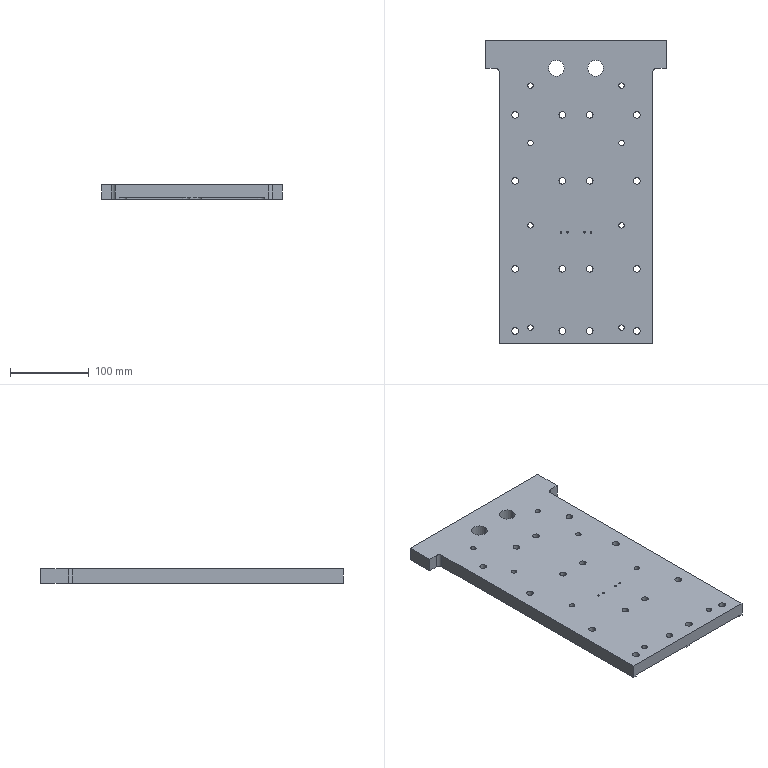CAM job | NX | 3-axis milling, drilling | part box 230 x 385 x 18 mm | stock box 234 x 389 x 18 mm
Tools:
number,name,description,diameter,corner_radius,flute_length,length,flutes
1,D6A45,Milling Tool-5 Parameters,6.0,0.0,50.0,75.0,2
6,6.8ZT,Drilling Tool,6.8,0.0,35.0,50.0,2
16,8.5ZT,Drilling Tool,8.5,0.0,35.0,50.0,2
15,D10,Milling Tool-5 Parameters,10.0,0.0,50.0,75.0,2
14,D10JING,Milling Tool-5 Parameters,10.0,0.0,50.0,75.0,2
Operations:
program,operation,operation_type,tool,method,geometry_group,spindle_rpm,surface_speed,feed_per_tooth,feed_cut,feed_plunge,cut_length_mm,path_length_mm,cut_time_min,machine_time_min
1,DRILLING,Operation,D6A45,METHOD,A,5000.0,94.0,0.035,350.0,0.0,104.0,1512.784,0.2971,0.438
1,DRILLING_COPY_COPY_COPY,Operation,6.8ZT,METHOD,A,2000.0,26.0,0.075,300.0,0.0,192.343,1184.008,0.6411,0.7403
1,DRILLING_COPY_COPY_COPY_COPY,Operation,8.5ZT,METHOD,A,2000.0,26.0,0.075,300.0,0.0,392.858,1786.981,1.31,1.449
1,ZLEVEL_PROFILE,ZLevelMilling,D10,METHOD,A,9500.0,298.0,0.1579,3000.0,1000.0,23943.971,24018.371,8.013,8.02
1,FLOOR_WALL,VolumeBased25DMillingOperation,D10,METHOD,A,9500.0,298.0,0.1579,3000.0,100.0,18551.401,18872.756,6.184,6.216
1,FLOOR_WALL_COPY,VolumeBased25DMillingOperation,D10JING,METHOD,A,9500.0,298.0,0.0789,1500.0,100.0,13092.07,13924.761,8.728,8.811
1,HOLE_MILLING,CylinderMilling,D10JING,METHOD,A,9500.0,298.0,0.1158,2200.0,100.0,1415.663,1620.663,0.6435,0.664
1,PLANAR_MILL_COPY_COPY_COPY,PlanarMilling,D6A45,METHOD,A,9500.0,179.0,0.0658,1250.0,100.0,2722.632,3148.624,2.178,2.221
1,FLOOR_WALL_COPY_COPY,VolumeBased25DMillingOperation,D10JING,METHOD,A,9500.0,298.0,0.0789,1500.0,100.0,1545.424,1781.436,1.03,1.054
1,PLANAR_MILL_COPY_COPY_COPY_COPY,PlanarMilling,D6A45,METHOD,A,9500.0,179.0,0.0658,1250.0,100.0,804.491,4092.329,0.6436,0.9724
1,ZLEVEL_PROFILE_COPY_1,ZLevelMilling,D10JING,METHOD,A,9500.0,298.0,0.0632,1200.0,1000.0,6318.112,6410.412,5.27,5.279